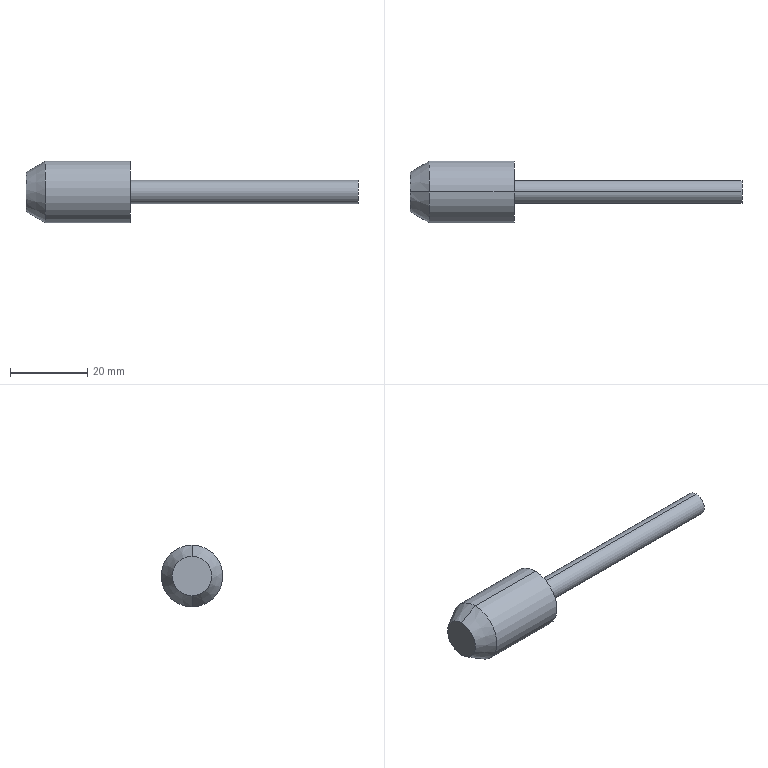Part | SolidWorks | features Revolution 1 | 1 solid | 9 faces | box 86 x 16 x 16 mm | volume 6778 mm3 | cylinder 4 | plane 3 | cone 2 | commonest cylinder face diameters 6 x2 16 x2
STEP:
#1=CARTESIAN_POINT('',(86.,0.,3.));
#2=VERTEX_POINT('',#1);
#3=CARTESIAN_POINT('',(86.,0.,-3.));
#4=VERTEX_POINT('',#3);
#5=CARTESIAN_POINT('',(86.,0.,0.));
#6=DIRECTION('',(-1.,0.,0.));
#7=DIRECTION('',(0.,0.,1.));
#8=AXIS2_PLACEMENT_3D('',#5,#6,#7);
#9=CIRCLE('',#8,3.);
#10=EDGE_CURVE('',#2,#4,#9,.T.);
#11=ORIENTED_EDGE('',*,*,#10,.T.);
#12=CARTESIAN_POINT('',(27.,0.,-3.));
#13=VERTEX_POINT('',#12);
#14=CARTESIAN_POINT('',(0.,0.,-3.));
#15=DIRECTION('',(-1.,0.,0.));
#16=VECTOR('',#15,1000.);
#17=LINE('',#14,#16);
#18=EDGE_CURVE('',#4,#13,#17,.T.);
#19=ORIENTED_EDGE('',*,*,#18,.T.);
#20=CARTESIAN_POINT('',(27.,0.,3.));
#21=VERTEX_POINT('',#20);
#22=CARTESIAN_POINT('',(27.,0.,0.));
#23=DIRECTION('',(-1.,0.,0.));
#24=DIRECTION('',(0.,0.,1.));
#25=AXIS2_PLACEMENT_3D('',#22,#23,#24);
#26=CIRCLE('',#25,3.);
#27=EDGE_CURVE('',#21,#13,#26,.T.);
#28=ORIENTED_EDGE('',*,*,#27,.F.);
#29=CARTESIAN_POINT('',(0.,0.,3.));
#30=DIRECTION('',(-1.,0.,0.));
#31=VECTOR('',#30,1000.);
#32=LINE('',#29,#31);
#33=EDGE_CURVE('',#2,#21,#32,.T.);
#34=ORIENTED_EDGE('',*,*,#33,.F.);
#35=EDGE_LOOP('',(#11,#19,#28,#34));
#36=FACE_OUTER_BOUND('',#35,.T.);
#37=CARTESIAN_POINT('',(0.,0.,0.));
#38=DIRECTION('',(-1.,0.,0.));
#39=DIRECTION('',(0.,0.,1.));
#40=AXIS2_PLACEMENT_3D('',#37,#38,#39);
#41=CYLINDRICAL_SURFACE('',#40,3.);
#42=ADVANCED_FACE('',(#36),#41,.T.);
#43=CARTESIAN_POINT('',(27.,0.,8.));
#44=VERTEX_POINT('',#43);
#45=CARTESIAN_POINT('',(27.,0.,-8.));
#46=VERTEX_POINT('',#45);
#47=CARTESIAN_POINT('',(27.,0.,0.));
#48=DIRECTION('',(-1.,0.,0.));
#49=DIRECTION('',(0.,0.,1.));
#50=AXIS2_PLACEMENT_3D('',#47,#48,#49);
#51=CIRCLE('',#50,8.);
#52=EDGE_CURVE('',#44,#46,#51,.T.);
#53=ORIENTED_EDGE('',*,*,#52,.T.);
#54=CARTESIAN_POINT('',(5.,0.,-8.));
#55=VERTEX_POINT('',#54);
#56=CARTESIAN_POINT('',(0.,0.,-8.));
#57=DIRECTION('',(-1.,0.,0.));
#58=VECTOR('',#57,1000.);
#59=LINE('',#56,#58);
#60=EDGE_CURVE('',#46,#55,#59,.T.);
#61=ORIENTED_EDGE('',*,*,#60,.T.);
#62=CARTESIAN_POINT('',(5.,0.,8.));
#63=VERTEX_POINT('',#62);
#64=CARTESIAN_POINT('',(5.,0.,0.));
#65=DIRECTION('',(-1.,0.,0.));
#66=DIRECTION('',(0.,0.,1.));
#67=AXIS2_PLACEMENT_3D('',#64,#65,#66);
#68=CIRCLE('',#67,8.);
#69=EDGE_CURVE('',#63,#55,#68,.T.);
#70=ORIENTED_EDGE('',*,*,#69,.F.);
#71=CARTESIAN_POINT('',(0.,0.,8.));
#72=DIRECTION('',(-1.,0.,0.));
#73=VECTOR('',#72,1000.);
#74=LINE('',#71,#73);
#75=EDGE_CURVE('',#44,#63,#74,.T.);
#76=ORIENTED_EDGE('',*,*,#75,.F.);
#77=EDGE_LOOP('',(#53,#61,#70,#76));
#78=FACE_OUTER_BOUND('',#77,.T.);
#79=CARTESIAN_POINT('',(0.,0.,0.));
#80=DIRECTION('',(-1.,0.,0.));
#81=DIRECTION('',(0.,0.,1.));
#82=AXIS2_PLACEMENT_3D('',#79,#80,#81);
#83=CYLINDRICAL_SURFACE('',#82,8.);
#84=ADVANCED_FACE('',(#78),#83,.T.);
#85=CARTESIAN_POINT('',(0.,0.,5.113));
#86=VERTEX_POINT('',#85);
#87=CARTESIAN_POINT('',(0.,0.,-5.113));
#88=VERTEX_POINT('',#87);
#89=CARTESIAN_POINT('',(0.,0.,0.));
#90=DIRECTION('',(-1.,0.,0.));
#91=DIRECTION('',(0.,0.,1.));
#92=AXIS2_PLACEMENT_3D('',#89,#90,#91);
#93=CIRCLE('',#92,5.113);
#94=EDGE_CURVE('',#86,#88,#93,.T.);
#95=ORIENTED_EDGE('',*,*,#94,.F.);
#96=CARTESIAN_POINT('',(5.,0.,8.));
#97=DIRECTION('',(0.866,0.,0.5));
#98=VECTOR('',#97,1000.);
#99=LINE('',#96,#98);
#100=EDGE_CURVE('',#86,#63,#99,.T.);
#101=ORIENTED_EDGE('',*,*,#100,.T.);
#102=ORIENTED_EDGE('',*,*,#69,.T.);
#103=CARTESIAN_POINT('',(5.,0.,-8.));
#104=DIRECTION('',(0.866,0.,-0.5));
#105=VECTOR('',#104,1000.);
#106=LINE('',#103,#105);
#107=EDGE_CURVE('',#88,#55,#106,.T.);
#108=ORIENTED_EDGE('',*,*,#107,.F.);
#109=EDGE_LOOP('',(#95,#101,#102,#108));
#110=FACE_OUTER_BOUND('',#109,.T.);
#111=CARTESIAN_POINT('',(5.,0.,0.));
#112=DIRECTION('',(1.,0.,0.));
#113=DIRECTION('',(0.,0.,-1.));
#114=AXIS2_PLACEMENT_3D('',#111,#112,#113);
#115=CONICAL_SURFACE('',#114,8.,0.5236);
#116=ADVANCED_FACE('',(#110),#115,.T.);
#117=CARTESIAN_POINT('',(0.,0.,0.));
#118=DIRECTION('',(-1.,0.,0.));
#119=DIRECTION('',(0.,0.,1.));
#120=AXIS2_PLACEMENT_3D('',#117,#118,#119);
#121=CIRCLE('',#120,5.113);
#122=EDGE_CURVE('',#88,#86,#121,.T.);
#123=ORIENTED_EDGE('',*,*,#122,.T.);
#124=ORIENTED_EDGE('',*,*,#94,.T.);
#125=EDGE_LOOP('',(#123,#124));
#126=FACE_OUTER_BOUND('',#125,.T.);
#127=CARTESIAN_POINT('',(0.,0.,0.));
#128=DIRECTION('',(1.,0.,0.));
#129=DIRECTION('',(0.,0.,-1.));
#130=AXIS2_PLACEMENT_3D('',#127,#128,#129);
#131=PLANE('',#130);
#132=ADVANCED_FACE('',(#126),#131,.F.);
#133=ORIENTED_EDGE('',*,*,#100,.F.);
#134=ORIENTED_EDGE('',*,*,#122,.F.);
#135=ORIENTED_EDGE('',*,*,#107,.T.);
#136=CARTESIAN_POINT('',(5.,0.,0.));
#137=DIRECTION('',(-1.,0.,0.));
#138=DIRECTION('',(0.,0.,1.));
#139=AXIS2_PLACEMENT_3D('',#136,#137,#138);
#140=CIRCLE('',#139,8.);
#141=EDGE_CURVE('',#55,#63,#140,.T.);
#142=ORIENTED_EDGE('',*,*,#141,.T.);
#143=EDGE_LOOP('',(#133,#134,#135,#142));
#144=FACE_OUTER_BOUND('',#143,.T.);
#145=CARTESIAN_POINT('',(5.,0.,0.));
#146=DIRECTION('',(1.,0.,0.));
#147=DIRECTION('',(0.,0.,-1.));
#148=AXIS2_PLACEMENT_3D('',#145,#146,#147);
#149=CONICAL_SURFACE('',#148,8.,0.5236);
#150=ADVANCED_FACE('',(#144),#149,.T.);
#151=ORIENTED_EDGE('',*,*,#60,.F.);
#152=CARTESIAN_POINT('',(27.,0.,0.));
#153=DIRECTION('',(-1.,0.,0.));
#154=DIRECTION('',(0.,0.,1.));
#155=AXIS2_PLACEMENT_3D('',#152,#153,#154);
#156=CIRCLE('',#155,8.);
#157=EDGE_CURVE('',#46,#44,#156,.T.);
#158=ORIENTED_EDGE('',*,*,#157,.T.);
#159=ORIENTED_EDGE('',*,*,#75,.T.);
#160=ORIENTED_EDGE('',*,*,#141,.F.);
#161=EDGE_LOOP('',(#151,#158,#159,#160));
#162=FACE_OUTER_BOUND('',#161,.T.);
#163=CARTESIAN_POINT('',(0.,0.,0.));
#164=DIRECTION('',(-1.,0.,0.));
#165=DIRECTION('',(0.,0.,1.));
#166=AXIS2_PLACEMENT_3D('',#163,#164,#165);
#167=CYLINDRICAL_SURFACE('',#166,8.);
#168=ADVANCED_FACE('',(#162),#167,.T.);
#169=ORIENTED_EDGE('',*,*,#52,.F.);
#170=ORIENTED_EDGE('',*,*,#157,.F.);
#171=EDGE_LOOP('',(#169,#170));
#172=FACE_OUTER_BOUND('',#171,.T.);
#173=ORIENTED_EDGE('',*,*,#27,.T.);
#174=CARTESIAN_POINT('',(27.,0.,0.));
#175=DIRECTION('',(-1.,0.,0.));
#176=DIRECTION('',(0.,0.,1.));
#177=AXIS2_PLACEMENT_3D('',#174,#175,#176);
#178=CIRCLE('',#177,3.);
#179=EDGE_CURVE('',#13,#21,#178,.T.);
#180=ORIENTED_EDGE('',*,*,#179,.T.);
#181=EDGE_LOOP('',(#173,#180));
#182=FACE_BOUND('',#181,.T.);
#183=CARTESIAN_POINT('',(27.,8.,0.));
#184=DIRECTION('',(-1.,0.,0.));
#185=DIRECTION('',(0.,0.,1.));
#186=AXIS2_PLACEMENT_3D('',#183,#184,#185);
#187=PLANE('',#186);
#188=ADVANCED_FACE('',(#172,#182),#187,.F.);
#189=ORIENTED_EDGE('',*,*,#18,.F.);
#190=CARTESIAN_POINT('',(86.,0.,0.));
#191=DIRECTION('',(-1.,0.,0.));
#192=DIRECTION('',(0.,0.,1.));
#193=AXIS2_PLACEMENT_3D('',#190,#191,#192);
#194=CIRCLE('',#193,3.);
#195=EDGE_CURVE('',#4,#2,#194,.T.);
#196=ORIENTED_EDGE('',*,*,#195,.T.);
#197=ORIENTED_EDGE('',*,*,#33,.T.);
#198=ORIENTED_EDGE('',*,*,#179,.F.);
#199=EDGE_LOOP('',(#189,#196,#197,#198));
#200=FACE_OUTER_BOUND('',#199,.T.);
#201=CARTESIAN_POINT('',(0.,0.,0.));
#202=DIRECTION('',(-1.,0.,0.));
#203=DIRECTION('',(0.,0.,1.));
#204=AXIS2_PLACEMENT_3D('',#201,#202,#203);
#205=CYLINDRICAL_SURFACE('',#204,3.);
#206=ADVANCED_FACE('',(#200),#205,.T.);
#207=ORIENTED_EDGE('',*,*,#10,.F.);
#208=ORIENTED_EDGE('',*,*,#195,.F.);
#209=EDGE_LOOP('',(#207,#208));
#210=FACE_OUTER_BOUND('',#209,.T.);
#211=CARTESIAN_POINT('',(86.,3.,0.));
#212=DIRECTION('',(-1.,0.,0.));
#213=DIRECTION('',(0.,0.,1.));
#214=AXIS2_PLACEMENT_3D('',#211,#212,#213);
#215=PLANE('',#214);
#216=ADVANCED_FACE('',(#210),#215,.F.);
#217=CLOSED_SHELL('',(#42,#84,#116,#132,#150,#168,#188,#206,#216));
#218=MANIFOLD_SOLID_BREP('',#217);
#219=CARTESIAN_POINT('',(0.,0.,0.));
#220=DIRECTION('',(0.,0.,1.));
#221=DIRECTION('',(1.,0.,0.));
#222=AXIS2_PLACEMENT_3D('',#219,#220,#221);
#223=(LENGTH_UNIT()NAMED_UNIT(*)SI_UNIT(.MILLI.,.METRE.));
#224=UNCERTAINTY_MEASURE_WITH_UNIT(LENGTH_MEASURE(0.00001),#223,'','');
#225=(NAMED_UNIT(*)PLANE_ANGLE_UNIT()SI_UNIT($,.RADIAN.));
#226=(NAMED_UNIT(*)SI_UNIT($,.STERADIAN.)SOLID_ANGLE_UNIT());
#227=(GEOMETRIC_REPRESENTATION_CONTEXT(3)GLOBAL_UNCERTAINTY_ASSIGNED_CONTEXT((#224))GLOBAL_UNIT_ASSIGNED_CONTEXT((#223,#225,#226))REPRESENTATION_CONTEXT('',''));
#228=ADVANCED_BREP_SHAPE_REPRESENTATION('',(#218,#222),#227);